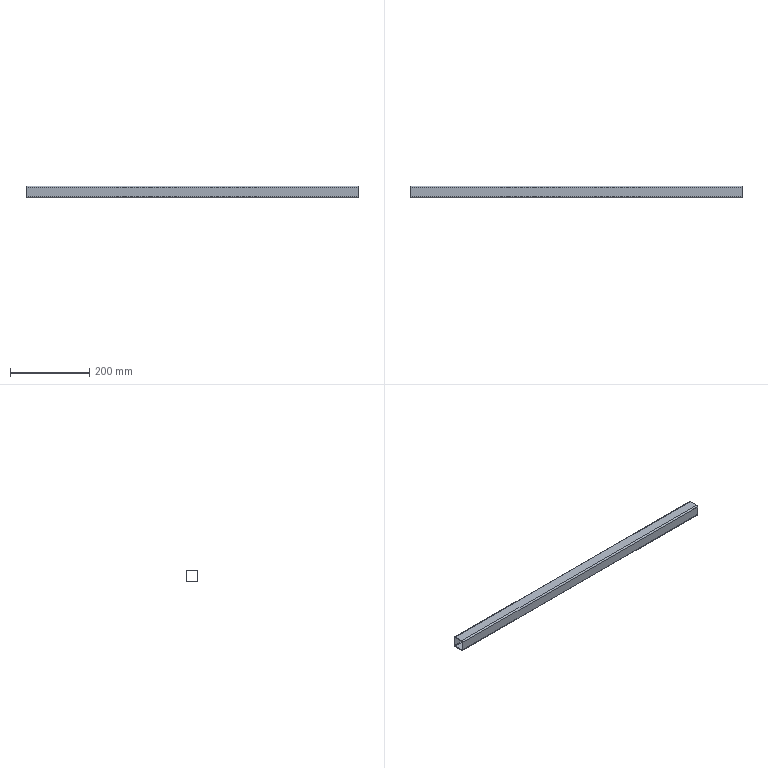Part | SolidWorks | features WeldMemberFeat 1, WeldmentFeature 1 | 1 solid | 18 faces | box 838 x 30 x 30 mm | volume 180231 mm3 | plane 10 | cylinder 8 | commonest cylinder face diameters 3.2 x4 7.2 x4
STEP:
#1=CARTESIAN_POINT('',(-419.,11.4,-15.));
#2=VERTEX_POINT('',#1);
#3=CARTESIAN_POINT('',(-419.,15.,-11.4));
#4=VERTEX_POINT('',#3);
#5=CARTESIAN_POINT('',(-419.,11.4,-11.4));
#6=DIRECTION('',(1.,0.,0.));
#7=DIRECTION('',(0.,0.,-1.));
#8=AXIS2_PLACEMENT_3D('',#5,#6,#7);
#9=CIRCLE('',#8,3.6);
#10=EDGE_CURVE('',#2,#4,#9,.T.);
#11=ORIENTED_EDGE('',*,*,#10,.T.);
#12=CARTESIAN_POINT('',(419.,15.,-11.4));
#13=VERTEX_POINT('',#12);
#14=CARTESIAN_POINT('',(419.,15.,-11.4));
#15=DIRECTION('',(-1.,0.,0.));
#16=VECTOR('',#15,1000.);
#17=LINE('',#14,#16);
#18=EDGE_CURVE('',#13,#4,#17,.T.);
#19=ORIENTED_EDGE('',*,*,#18,.F.);
#20=CARTESIAN_POINT('',(419.,11.4,-15.));
#21=VERTEX_POINT('',#20);
#22=CARTESIAN_POINT('',(419.,11.4,-11.4));
#23=DIRECTION('',(1.,0.,0.));
#24=DIRECTION('',(0.,0.,-1.));
#25=AXIS2_PLACEMENT_3D('',#22,#23,#24);
#26=CIRCLE('',#25,3.6);
#27=EDGE_CURVE('',#21,#13,#26,.T.);
#28=ORIENTED_EDGE('',*,*,#27,.F.);
#29=CARTESIAN_POINT('',(419.,11.4,-15.));
#30=DIRECTION('',(-1.,0.,0.));
#31=VECTOR('',#30,1000.);
#32=LINE('',#29,#31);
#33=EDGE_CURVE('',#21,#2,#32,.T.);
#34=ORIENTED_EDGE('',*,*,#33,.T.);
#35=EDGE_LOOP('',(#11,#19,#28,#34));
#36=FACE_OUTER_BOUND('',#35,.T.);
#37=CARTESIAN_POINT('',(419.,11.4,-11.4));
#38=DIRECTION('',(-1.,0.,0.));
#39=DIRECTION('',(0.,0.,1.));
#40=AXIS2_PLACEMENT_3D('',#37,#38,#39);
#41=CYLINDRICAL_SURFACE('',#40,3.6);
#42=ADVANCED_FACE('',(#36),#41,.T.);
#43=CARTESIAN_POINT('',(-419.,15.,11.4));
#44=VERTEX_POINT('',#43);
#45=CARTESIAN_POINT('',(-419.,15.,-11.4));
#46=DIRECTION('',(0.,0.,1.));
#47=VECTOR('',#46,1000.);
#48=LINE('',#45,#47);
#49=EDGE_CURVE('',#4,#44,#48,.T.);
#50=ORIENTED_EDGE('',*,*,#49,.T.);
#51=CARTESIAN_POINT('',(419.,15.,11.4));
#52=VERTEX_POINT('',#51);
#53=CARTESIAN_POINT('',(419.,15.,11.4));
#54=DIRECTION('',(-1.,0.,0.));
#55=VECTOR('',#54,1000.);
#56=LINE('',#53,#55);
#57=EDGE_CURVE('',#52,#44,#56,.T.);
#58=ORIENTED_EDGE('',*,*,#57,.F.);
#59=CARTESIAN_POINT('',(419.,15.,-11.4));
#60=DIRECTION('',(0.,0.,1.));
#61=VECTOR('',#60,1000.);
#62=LINE('',#59,#61);
#63=EDGE_CURVE('',#13,#52,#62,.T.);
#64=ORIENTED_EDGE('',*,*,#63,.F.);
#65=ORIENTED_EDGE('',*,*,#18,.T.);
#66=EDGE_LOOP('',(#50,#58,#64,#65));
#67=FACE_OUTER_BOUND('',#66,.T.);
#68=CARTESIAN_POINT('',(419.,15.,-11.4));
#69=DIRECTION('',(0.,-1.,0.));
#70=DIRECTION('',(0.,0.,-1.));
#71=AXIS2_PLACEMENT_3D('',#68,#69,#70);
#72=PLANE('',#71);
#73=ADVANCED_FACE('',(#67),#72,.F.);
#74=CARTESIAN_POINT('',(-419.,11.4,15.));
#75=VERTEX_POINT('',#74);
#76=CARTESIAN_POINT('',(-419.,11.4,11.4));
#77=DIRECTION('',(1.,0.,0.));
#78=DIRECTION('',(0.,0.,-1.));
#79=AXIS2_PLACEMENT_3D('',#76,#77,#78);
#80=CIRCLE('',#79,3.6);
#81=EDGE_CURVE('',#44,#75,#80,.T.);
#82=ORIENTED_EDGE('',*,*,#81,.T.);
#83=CARTESIAN_POINT('',(419.,11.4,15.));
#84=VERTEX_POINT('',#83);
#85=CARTESIAN_POINT('',(419.,11.4,15.));
#86=DIRECTION('',(-1.,0.,0.));
#87=VECTOR('',#86,1000.);
#88=LINE('',#85,#87);
#89=EDGE_CURVE('',#84,#75,#88,.T.);
#90=ORIENTED_EDGE('',*,*,#89,.F.);
#91=CARTESIAN_POINT('',(419.,11.4,11.4));
#92=DIRECTION('',(1.,0.,0.));
#93=DIRECTION('',(0.,0.,-1.));
#94=AXIS2_PLACEMENT_3D('',#91,#92,#93);
#95=CIRCLE('',#94,3.6);
#96=EDGE_CURVE('',#52,#84,#95,.T.);
#97=ORIENTED_EDGE('',*,*,#96,.F.);
#98=ORIENTED_EDGE('',*,*,#57,.T.);
#99=EDGE_LOOP('',(#82,#90,#97,#98));
#100=FACE_OUTER_BOUND('',#99,.T.);
#101=CARTESIAN_POINT('',(419.,11.4,11.4));
#102=DIRECTION('',(-1.,0.,0.));
#103=DIRECTION('',(0.,0.,1.));
#104=AXIS2_PLACEMENT_3D('',#101,#102,#103);
#105=CYLINDRICAL_SURFACE('',#104,3.6);
#106=ADVANCED_FACE('',(#100),#105,.T.);
#107=CARTESIAN_POINT('',(-419.,-11.4,15.));
#108=VERTEX_POINT('',#107);
#109=CARTESIAN_POINT('',(-419.,-11.4,15.));
#110=DIRECTION('',(0.,-1.,0.));
#111=VECTOR('',#110,1000.);
#112=LINE('',#109,#111);
#113=EDGE_CURVE('',#75,#108,#112,.T.);
#114=ORIENTED_EDGE('',*,*,#113,.T.);
#115=CARTESIAN_POINT('',(419.,-11.4,15.));
#116=VERTEX_POINT('',#115);
#117=CARTESIAN_POINT('',(419.,-11.4,15.));
#118=DIRECTION('',(-1.,0.,0.));
#119=VECTOR('',#118,1000.);
#120=LINE('',#117,#119);
#121=EDGE_CURVE('',#116,#108,#120,.T.);
#122=ORIENTED_EDGE('',*,*,#121,.F.);
#123=CARTESIAN_POINT('',(419.,-11.4,15.));
#124=DIRECTION('',(0.,-1.,0.));
#125=VECTOR('',#124,1000.);
#126=LINE('',#123,#125);
#127=EDGE_CURVE('',#84,#116,#126,.T.);
#128=ORIENTED_EDGE('',*,*,#127,.F.);
#129=ORIENTED_EDGE('',*,*,#89,.T.);
#130=EDGE_LOOP('',(#114,#122,#128,#129));
#131=FACE_OUTER_BOUND('',#130,.T.);
#132=CARTESIAN_POINT('',(419.,-11.4,15.));
#133=DIRECTION('',(0.,0.,-1.));
#134=DIRECTION('',(-1.,0.,0.));
#135=AXIS2_PLACEMENT_3D('',#132,#133,#134);
#136=PLANE('',#135);
#137=ADVANCED_FACE('',(#131),#136,.F.);
#138=CARTESIAN_POINT('',(-419.,-15.,11.4));
#139=VERTEX_POINT('',#138);
#140=CARTESIAN_POINT('',(-419.,-11.4,11.4));
#141=DIRECTION('',(1.,0.,0.));
#142=DIRECTION('',(0.,0.,-1.));
#143=AXIS2_PLACEMENT_3D('',#140,#141,#142);
#144=CIRCLE('',#143,3.6);
#145=EDGE_CURVE('',#108,#139,#144,.T.);
#146=ORIENTED_EDGE('',*,*,#145,.T.);
#147=CARTESIAN_POINT('',(419.,-15.,11.4));
#148=VERTEX_POINT('',#147);
#149=CARTESIAN_POINT('',(419.,-15.,11.4));
#150=DIRECTION('',(-1.,0.,0.));
#151=VECTOR('',#150,1000.);
#152=LINE('',#149,#151);
#153=EDGE_CURVE('',#148,#139,#152,.T.);
#154=ORIENTED_EDGE('',*,*,#153,.F.);
#155=CARTESIAN_POINT('',(419.,-11.4,11.4));
#156=DIRECTION('',(1.,0.,0.));
#157=DIRECTION('',(0.,0.,-1.));
#158=AXIS2_PLACEMENT_3D('',#155,#156,#157);
#159=CIRCLE('',#158,3.6);
#160=EDGE_CURVE('',#116,#148,#159,.T.);
#161=ORIENTED_EDGE('',*,*,#160,.F.);
#162=ORIENTED_EDGE('',*,*,#121,.T.);
#163=EDGE_LOOP('',(#146,#154,#161,#162));
#164=FACE_OUTER_BOUND('',#163,.T.);
#165=CARTESIAN_POINT('',(419.,-11.4,11.4));
#166=DIRECTION('',(-1.,0.,0.));
#167=DIRECTION('',(0.,0.,1.));
#168=AXIS2_PLACEMENT_3D('',#165,#166,#167);
#169=CYLINDRICAL_SURFACE('',#168,3.6);
#170=ADVANCED_FACE('',(#164),#169,.T.);
#171=CARTESIAN_POINT('',(-419.,-15.,-11.4));
#172=VERTEX_POINT('',#171);
#173=CARTESIAN_POINT('',(-419.,-15.,11.4));
#174=DIRECTION('',(0.,0.,-1.));
#175=VECTOR('',#174,1000.);
#176=LINE('',#173,#175);
#177=EDGE_CURVE('',#139,#172,#176,.T.);
#178=ORIENTED_EDGE('',*,*,#177,.T.);
#179=CARTESIAN_POINT('',(419.,-15.,-11.4));
#180=VERTEX_POINT('',#179);
#181=CARTESIAN_POINT('',(419.,-15.,-11.4));
#182=DIRECTION('',(-1.,0.,0.));
#183=VECTOR('',#182,1000.);
#184=LINE('',#181,#183);
#185=EDGE_CURVE('',#180,#172,#184,.T.);
#186=ORIENTED_EDGE('',*,*,#185,.F.);
#187=CARTESIAN_POINT('',(419.,-15.,11.4));
#188=DIRECTION('',(0.,0.,-1.));
#189=VECTOR('',#188,1000.);
#190=LINE('',#187,#189);
#191=EDGE_CURVE('',#148,#180,#190,.T.);
#192=ORIENTED_EDGE('',*,*,#191,.F.);
#193=ORIENTED_EDGE('',*,*,#153,.T.);
#194=EDGE_LOOP('',(#178,#186,#192,#193));
#195=FACE_OUTER_BOUND('',#194,.T.);
#196=CARTESIAN_POINT('',(419.,-15.,11.4));
#197=DIRECTION('',(0.,1.,0.));
#198=DIRECTION('',(0.,0.,1.));
#199=AXIS2_PLACEMENT_3D('',#196,#197,#198);
#200=PLANE('',#199);
#201=ADVANCED_FACE('',(#195),#200,.F.);
#202=CARTESIAN_POINT('',(-419.,-11.4,-15.));
#203=VERTEX_POINT('',#202);
#204=CARTESIAN_POINT('',(-419.,-11.4,-11.4));
#205=DIRECTION('',(1.,0.,0.));
#206=DIRECTION('',(0.,0.,-1.));
#207=AXIS2_PLACEMENT_3D('',#204,#205,#206);
#208=CIRCLE('',#207,3.6);
#209=EDGE_CURVE('',#172,#203,#208,.T.);
#210=ORIENTED_EDGE('',*,*,#209,.T.);
#211=CARTESIAN_POINT('',(419.,-11.4,-15.));
#212=VERTEX_POINT('',#211);
#213=CARTESIAN_POINT('',(419.,-11.4,-15.));
#214=DIRECTION('',(-1.,0.,0.));
#215=VECTOR('',#214,1000.);
#216=LINE('',#213,#215);
#217=EDGE_CURVE('',#212,#203,#216,.T.);
#218=ORIENTED_EDGE('',*,*,#217,.F.);
#219=CARTESIAN_POINT('',(419.,-11.4,-11.4));
#220=DIRECTION('',(1.,0.,0.));
#221=DIRECTION('',(0.,0.,-1.));
#222=AXIS2_PLACEMENT_3D('',#219,#220,#221);
#223=CIRCLE('',#222,3.6);
#224=EDGE_CURVE('',#180,#212,#223,.T.);
#225=ORIENTED_EDGE('',*,*,#224,.F.);
#226=ORIENTED_EDGE('',*,*,#185,.T.);
#227=EDGE_LOOP('',(#210,#218,#225,#226));
#228=FACE_OUTER_BOUND('',#227,.T.);
#229=CARTESIAN_POINT('',(419.,-11.4,-11.4));
#230=DIRECTION('',(-1.,0.,0.));
#231=DIRECTION('',(0.,0.,1.));
#232=AXIS2_PLACEMENT_3D('',#229,#230,#231);
#233=CYLINDRICAL_SURFACE('',#232,3.6);
#234=ADVANCED_FACE('',(#228),#233,.T.);
#235=CARTESIAN_POINT('',(-419.,13.,11.4));
#236=VERTEX_POINT('',#235);
#237=CARTESIAN_POINT('',(-419.,11.4,13.));
#238=VERTEX_POINT('',#237);
#239=CARTESIAN_POINT('',(-419.,11.4,11.4));
#240=DIRECTION('',(1.,0.,0.));
#241=DIRECTION('',(0.,0.,-1.));
#242=AXIS2_PLACEMENT_3D('',#239,#240,#241);
#243=CIRCLE('',#242,1.6);
#244=EDGE_CURVE('',#236,#238,#243,.T.);
#245=ORIENTED_EDGE('',*,*,#244,.F.);
#246=CARTESIAN_POINT('',(419.,13.,11.4));
#247=VERTEX_POINT('',#246);
#248=CARTESIAN_POINT('',(419.,13.,11.4));
#249=DIRECTION('',(-1.,0.,0.));
#250=VECTOR('',#249,1000.);
#251=LINE('',#248,#250);
#252=EDGE_CURVE('',#247,#236,#251,.T.);
#253=ORIENTED_EDGE('',*,*,#252,.F.);
#254=CARTESIAN_POINT('',(419.,11.4,13.));
#255=VERTEX_POINT('',#254);
#256=CARTESIAN_POINT('',(419.,11.4,11.4));
#257=DIRECTION('',(1.,0.,0.));
#258=DIRECTION('',(0.,0.,-1.));
#259=AXIS2_PLACEMENT_3D('',#256,#257,#258);
#260=CIRCLE('',#259,1.6);
#261=EDGE_CURVE('',#247,#255,#260,.T.);
#262=ORIENTED_EDGE('',*,*,#261,.T.);
#263=CARTESIAN_POINT('',(419.,11.4,13.));
#264=DIRECTION('',(-1.,0.,0.));
#265=VECTOR('',#264,1000.);
#266=LINE('',#263,#265);
#267=EDGE_CURVE('',#255,#238,#266,.T.);
#268=ORIENTED_EDGE('',*,*,#267,.T.);
#269=EDGE_LOOP('',(#245,#253,#262,#268));
#270=FACE_OUTER_BOUND('',#269,.T.);
#271=CARTESIAN_POINT('',(419.,11.4,11.4));
#272=DIRECTION('',(-1.,0.,0.));
#273=DIRECTION('',(0.,0.,1.));
#274=AXIS2_PLACEMENT_3D('',#271,#272,#273);
#275=CYLINDRICAL_SURFACE('',#274,1.6);
#276=ADVANCED_FACE('',(#270),#275,.F.);
#277=CARTESIAN_POINT('',(-419.,13.,-11.4));
#278=VERTEX_POINT('',#277);
#279=CARTESIAN_POINT('',(-419.,13.,-11.4));
#280=DIRECTION('',(0.,0.,1.));
#281=VECTOR('',#280,1000.);
#282=LINE('',#279,#281);
#283=EDGE_CURVE('',#278,#236,#282,.T.);
#284=ORIENTED_EDGE('',*,*,#283,.F.);
#285=CARTESIAN_POINT('',(419.,13.,-11.4));
#286=VERTEX_POINT('',#285);
#287=CARTESIAN_POINT('',(419.,13.,-11.4));
#288=DIRECTION('',(-1.,0.,0.));
#289=VECTOR('',#288,1000.);
#290=LINE('',#287,#289);
#291=EDGE_CURVE('',#286,#278,#290,.T.);
#292=ORIENTED_EDGE('',*,*,#291,.F.);
#293=CARTESIAN_POINT('',(419.,13.,-11.4));
#294=DIRECTION('',(0.,0.,1.));
#295=VECTOR('',#294,1000.);
#296=LINE('',#293,#295);
#297=EDGE_CURVE('',#286,#247,#296,.T.);
#298=ORIENTED_EDGE('',*,*,#297,.T.);
#299=ORIENTED_EDGE('',*,*,#252,.T.);
#300=EDGE_LOOP('',(#284,#292,#298,#299));
#301=FACE_OUTER_BOUND('',#300,.T.);
#302=CARTESIAN_POINT('',(419.,13.,-11.4));
#303=DIRECTION('',(0.,-1.,0.));
#304=DIRECTION('',(0.,0.,-1.));
#305=AXIS2_PLACEMENT_3D('',#302,#303,#304);
#306=PLANE('',#305);
#307=ADVANCED_FACE('',(#301),#306,.T.);
#308=CARTESIAN_POINT('',(-419.,11.4,-13.));
#309=VERTEX_POINT('',#308);
#310=CARTESIAN_POINT('',(-419.,11.4,-11.4));
#311=DIRECTION('',(1.,0.,0.));
#312=DIRECTION('',(0.,0.,-1.));
#313=AXIS2_PLACEMENT_3D('',#310,#311,#312);
#314=CIRCLE('',#313,1.6);
#315=EDGE_CURVE('',#309,#278,#314,.T.);
#316=ORIENTED_EDGE('',*,*,#315,.F.);
#317=CARTESIAN_POINT('',(419.,11.4,-13.));
#318=VERTEX_POINT('',#317);
#319=CARTESIAN_POINT('',(419.,11.4,-13.));
#320=DIRECTION('',(-1.,0.,0.));
#321=VECTOR('',#320,1000.);
#322=LINE('',#319,#321);
#323=EDGE_CURVE('',#318,#309,#322,.T.);
#324=ORIENTED_EDGE('',*,*,#323,.F.);
#325=CARTESIAN_POINT('',(419.,11.4,-11.4));
#326=DIRECTION('',(1.,0.,0.));
#327=DIRECTION('',(0.,0.,-1.));
#328=AXIS2_PLACEMENT_3D('',#325,#326,#327);
#329=CIRCLE('',#328,1.6);
#330=EDGE_CURVE('',#318,#286,#329,.T.);
#331=ORIENTED_EDGE('',*,*,#330,.T.);
#332=ORIENTED_EDGE('',*,*,#291,.T.);
#333=EDGE_LOOP('',(#316,#324,#331,#332));
#334=FACE_OUTER_BOUND('',#333,.T.);
#335=CARTESIAN_POINT('',(419.,11.4,-11.4));
#336=DIRECTION('',(-1.,0.,0.));
#337=DIRECTION('',(0.,0.,1.));
#338=AXIS2_PLACEMENT_3D('',#335,#336,#337);
#339=CYLINDRICAL_SURFACE('',#338,1.6);
#340=ADVANCED_FACE('',(#334),#339,.F.);
#341=CARTESIAN_POINT('',(-419.,-11.4,-13.));
#342=VERTEX_POINT('',#341);
#343=CARTESIAN_POINT('',(-419.,11.4,-13.));
#344=DIRECTION('',(0.,1.,0.));
#345=VECTOR('',#344,1000.);
#346=LINE('',#343,#345);
#347=EDGE_CURVE('',#342,#309,#346,.T.);
#348=ORIENTED_EDGE('',*,*,#347,.F.);
#349=CARTESIAN_POINT('',(419.,-11.4,-13.));
#350=VERTEX_POINT('',#349);
#351=CARTESIAN_POINT('',(419.,-11.4,-13.));
#352=DIRECTION('',(-1.,0.,0.));
#353=VECTOR('',#352,1000.);
#354=LINE('',#351,#353);
#355=EDGE_CURVE('',#350,#342,#354,.T.);
#356=ORIENTED_EDGE('',*,*,#355,.F.);
#357=CARTESIAN_POINT('',(419.,11.4,-13.));
#358=DIRECTION('',(0.,1.,0.));
#359=VECTOR('',#358,1000.);
#360=LINE('',#357,#359);
#361=EDGE_CURVE('',#350,#318,#360,.T.);
#362=ORIENTED_EDGE('',*,*,#361,.T.);
#363=ORIENTED_EDGE('',*,*,#323,.T.);
#364=EDGE_LOOP('',(#348,#356,#362,#363));
#365=FACE_OUTER_BOUND('',#364,.T.);
#366=CARTESIAN_POINT('',(419.,11.4,-13.));
#367=DIRECTION('',(0.,0.,1.));
#368=DIRECTION('',(1.,0.,0.));
#369=AXIS2_PLACEMENT_3D('',#366,#367,#368);
#370=PLANE('',#369);
#371=ADVANCED_FACE('',(#365),#370,.T.);
#372=CARTESIAN_POINT('',(-419.,-13.,-11.4));
#373=VERTEX_POINT('',#372);
#374=CARTESIAN_POINT('',(-419.,-11.4,-11.4));
#375=DIRECTION('',(1.,0.,0.));
#376=DIRECTION('',(0.,0.,-1.));
#377=AXIS2_PLACEMENT_3D('',#374,#375,#376);
#378=CIRCLE('',#377,1.6);
#379=EDGE_CURVE('',#373,#342,#378,.T.);
#380=ORIENTED_EDGE('',*,*,#379,.F.);
#381=CARTESIAN_POINT('',(419.,-13.,-11.4));
#382=VERTEX_POINT('',#381);
#383=CARTESIAN_POINT('',(419.,-13.,-11.4));
#384=DIRECTION('',(-1.,0.,0.));
#385=VECTOR('',#384,1000.);
#386=LINE('',#383,#385);
#387=EDGE_CURVE('',#382,#373,#386,.T.);
#388=ORIENTED_EDGE('',*,*,#387,.F.);
#389=CARTESIAN_POINT('',(419.,-11.4,-11.4));
#390=DIRECTION('',(1.,0.,0.));
#391=DIRECTION('',(0.,0.,-1.));
#392=AXIS2_PLACEMENT_3D('',#389,#390,#391);
#393=CIRCLE('',#392,1.6);
#394=EDGE_CURVE('',#382,#350,#393,.T.);
#395=ORIENTED_EDGE('',*,*,#394,.T.);
#396=ORIENTED_EDGE('',*,*,#355,.T.);
#397=EDGE_LOOP('',(#380,#388,#395,#396));
#398=FACE_OUTER_BOUND('',#397,.T.);
#399=CARTESIAN_POINT('',(419.,-11.4,-11.4));
#400=DIRECTION('',(-1.,0.,0.));
#401=DIRECTION('',(0.,0.,1.));
#402=AXIS2_PLACEMENT_3D('',#399,#400,#401);
#403=CYLINDRICAL_SURFACE('',#402,1.6);
#404=ADVANCED_FACE('',(#398),#403,.F.);
#405=CARTESIAN_POINT('',(-419.,-13.,11.4));
#406=VERTEX_POINT('',#405);
#407=CARTESIAN_POINT('',(-419.,-13.,11.4));
#408=DIRECTION('',(0.,0.,-1.));
#409=VECTOR('',#408,1000.);
#410=LINE('',#407,#409);
#411=EDGE_CURVE('',#406,#373,#410,.T.);
#412=ORIENTED_EDGE('',*,*,#411,.F.);
#413=CARTESIAN_POINT('',(419.,-13.,11.4));
#414=VERTEX_POINT('',#413);
#415=CARTESIAN_POINT('',(419.,-13.,11.4));
#416=DIRECTION('',(-1.,0.,0.));
#417=VECTOR('',#416,1000.);
#418=LINE('',#415,#417);
#419=EDGE_CURVE('',#414,#406,#418,.T.);
#420=ORIENTED_EDGE('',*,*,#419,.F.);
#421=CARTESIAN_POINT('',(419.,-13.,11.4));
#422=DIRECTION('',(0.,0.,-1.));
#423=VECTOR('',#422,1000.);
#424=LINE('',#421,#423);
#425=EDGE_CURVE('',#414,#382,#424,.T.);
#426=ORIENTED_EDGE('',*,*,#425,.T.);
#427=ORIENTED_EDGE('',*,*,#387,.T.);
#428=EDGE_LOOP('',(#412,#420,#426,#427));
#429=FACE_OUTER_BOUND('',#428,.T.);
#430=CARTESIAN_POINT('',(419.,-13.,11.4));
#431=DIRECTION('',(0.,1.,0.));
#432=DIRECTION('',(0.,0.,1.));
#433=AXIS2_PLACEMENT_3D('',#430,#431,#432);
#434=PLANE('',#433);
#435=ADVANCED_FACE('',(#429),#434,.T.);
#436=CARTESIAN_POINT('',(-419.,-11.4,13.));
#437=VERTEX_POINT('',#436);
#438=CARTESIAN_POINT('',(-419.,-11.4,11.4));
#439=DIRECTION('',(1.,0.,0.));
#440=DIRECTION('',(0.,0.,-1.));
#441=AXIS2_PLACEMENT_3D('',#438,#439,#440);
#442=CIRCLE('',#441,1.6);
#443=EDGE_CURVE('',#437,#406,#442,.T.);
#444=ORIENTED_EDGE('',*,*,#443,.F.);
#445=CARTESIAN_POINT('',(419.,-11.4,13.));
#446=VERTEX_POINT('',#445);
#447=CARTESIAN_POINT('',(419.,-11.4,13.));
#448=DIRECTION('',(-1.,0.,0.));
#449=VECTOR('',#448,1000.);
#450=LINE('',#447,#449);
#451=EDGE_CURVE('',#446,#437,#450,.T.);
#452=ORIENTED_EDGE('',*,*,#451,.F.);
#453=CARTESIAN_POINT('',(419.,-11.4,11.4));
#454=DIRECTION('',(1.,0.,0.));
#455=DIRECTION('',(0.,0.,-1.));
#456=AXIS2_PLACEMENT_3D('',#453,#454,#455);
#457=CIRCLE('',#456,1.6);
#458=EDGE_CURVE('',#446,#414,#457,.T.);
#459=ORIENTED_EDGE('',*,*,#458,.T.);
#460=ORIENTED_EDGE('',*,*,#419,.T.);
#461=EDGE_LOOP('',(#444,#452,#459,#460));
#462=FACE_OUTER_BOUND('',#461,.T.);
#463=CARTESIAN_POINT('',(419.,-11.4,11.4));
#464=DIRECTION('',(-1.,0.,0.));
#465=DIRECTION('',(0.,0.,1.));
#466=AXIS2_PLACEMENT_3D('',#463,#464,#465);
#467=CYLINDRICAL_SURFACE('',#466,1.6);
#468=ADVANCED_FACE('',(#462),#467,.F.);
#469=CARTESIAN_POINT('',(-419.,-11.4,13.));
#470=DIRECTION('',(0.,-1.,0.));
#471=VECTOR('',#470,1000.);
#472=LINE('',#469,#471);
#473=EDGE_CURVE('',#238,#437,#472,.T.);
#474=ORIENTED_EDGE('',*,*,#473,.F.);
#475=ORIENTED_EDGE('',*,*,#267,.F.);
#476=CARTESIAN_POINT('',(419.,-11.4,13.));
#477=DIRECTION('',(0.,-1.,0.));
#478=VECTOR('',#477,1000.);
#479=LINE('',#476,#478);
#480=EDGE_CURVE('',#255,#446,#479,.T.);
#481=ORIENTED_EDGE('',*,*,#480,.T.);
#482=ORIENTED_EDGE('',*,*,#451,.T.);
#483=EDGE_LOOP('',(#474,#475,#481,#482));
#484=FACE_OUTER_BOUND('',#483,.T.);
#485=CARTESIAN_POINT('',(419.,-11.4,13.));
#486=DIRECTION('',(0.,0.,-1.));
#487=DIRECTION('',(-1.,0.,0.));
#488=AXIS2_PLACEMENT_3D('',#485,#486,#487);
#489=PLANE('',#488);
#490=ADVANCED_FACE('',(#484),#489,.T.);
#491=CARTESIAN_POINT('',(-419.,11.4,-15.));
#492=DIRECTION('',(0.,1.,0.));
#493=VECTOR('',#492,1000.);
#494=LINE('',#491,#493);
#495=EDGE_CURVE('',#203,#2,#494,.T.);
#496=ORIENTED_EDGE('',*,*,#495,.T.);
#497=ORIENTED_EDGE('',*,*,#33,.F.);
#498=CARTESIAN_POINT('',(419.,11.4,-15.));
#499=DIRECTION('',(0.,1.,0.));
#500=VECTOR('',#499,1000.);
#501=LINE('',#498,#500);
#502=EDGE_CURVE('',#212,#21,#501,.T.);
#503=ORIENTED_EDGE('',*,*,#502,.F.);
#504=ORIENTED_EDGE('',*,*,#217,.T.);
#505=EDGE_LOOP('',(#496,#497,#503,#504));
#506=FACE_OUTER_BOUND('',#505,.T.);
#507=CARTESIAN_POINT('',(419.,11.4,-15.));
#508=DIRECTION('',(0.,0.,1.));
#509=DIRECTION('',(1.,0.,0.));
#510=AXIS2_PLACEMENT_3D('',#507,#508,#509);
#511=PLANE('',#510);
#512=ADVANCED_FACE('',(#506),#511,.F.);
#513=ORIENTED_EDGE('',*,*,#261,.F.);
#514=ORIENTED_EDGE('',*,*,#297,.F.);
#515=ORIENTED_EDGE('',*,*,#330,.F.);
#516=ORIENTED_EDGE('',*,*,#361,.F.);
#517=ORIENTED_EDGE('',*,*,#394,.F.);
#518=ORIENTED_EDGE('',*,*,#425,.F.);
#519=ORIENTED_EDGE('',*,*,#458,.F.);
#520=ORIENTED_EDGE('',*,*,#480,.F.);
#521=EDGE_LOOP('',(#513,#514,#515,#516,#517,#518,#519,#520));
#522=FACE_BOUND('',#521,.T.);
#523=ORIENTED_EDGE('',*,*,#27,.T.);
#524=ORIENTED_EDGE('',*,*,#63,.T.);
#525=ORIENTED_EDGE('',*,*,#96,.T.);
#526=ORIENTED_EDGE('',*,*,#127,.T.);
#527=ORIENTED_EDGE('',*,*,#160,.T.);
#528=ORIENTED_EDGE('',*,*,#191,.T.);
#529=ORIENTED_EDGE('',*,*,#224,.T.);
#530=ORIENTED_EDGE('',*,*,#502,.T.);
#531=EDGE_LOOP('',(#523,#524,#525,#526,#527,#528,#529,#530));
#532=FACE_OUTER_BOUND('',#531,.T.);
#533=CARTESIAN_POINT('',(419.,11.4,-11.4));
#534=DIRECTION('',(1.,0.,0.));
#535=DIRECTION('',(0.,0.,-1.));
#536=AXIS2_PLACEMENT_3D('',#533,#534,#535);
#537=PLANE('',#536);
#538=ADVANCED_FACE('',(#522,#532),#537,.T.);
#539=ORIENTED_EDGE('',*,*,#244,.T.);
#540=ORIENTED_EDGE('',*,*,#473,.T.);
#541=ORIENTED_EDGE('',*,*,#443,.T.);
#542=ORIENTED_EDGE('',*,*,#411,.T.);
#543=ORIENTED_EDGE('',*,*,#379,.T.);
#544=ORIENTED_EDGE('',*,*,#347,.T.);
#545=ORIENTED_EDGE('',*,*,#315,.T.);
#546=ORIENTED_EDGE('',*,*,#283,.T.);
#547=EDGE_LOOP('',(#539,#540,#541,#542,#543,#544,#545,#546));
#548=FACE_BOUND('',#547,.T.);
#549=ORIENTED_EDGE('',*,*,#10,.F.);
#550=ORIENTED_EDGE('',*,*,#495,.F.);
#551=ORIENTED_EDGE('',*,*,#209,.F.);
#552=ORIENTED_EDGE('',*,*,#177,.F.);
#553=ORIENTED_EDGE('',*,*,#145,.F.);
#554=ORIENTED_EDGE('',*,*,#113,.F.);
#555=ORIENTED_EDGE('',*,*,#81,.F.);
#556=ORIENTED_EDGE('',*,*,#49,.F.);
#557=EDGE_LOOP('',(#549,#550,#551,#552,#553,#554,#555,#556));
#558=FACE_OUTER_BOUND('',#557,.T.);
#559=CARTESIAN_POINT('',(-419.,11.4,-11.4));
#560=DIRECTION('',(1.,0.,0.));
#561=DIRECTION('',(0.,0.,-1.));
#562=AXIS2_PLACEMENT_3D('',#559,#560,#561);
#563=PLANE('',#562);
#564=ADVANCED_FACE('',(#548,#558),#563,.F.);
#565=CLOSED_SHELL('',(#42,#73,#106,#137,#170,#201,#234,#276,#307,#340,#371,#404,#435,#468,#490,#512,#538,#564));
#566=MANIFOLD_SOLID_BREP('',#565);
#567=CARTESIAN_POINT('',(0.,0.,0.));
#568=DIRECTION('',(0.,0.,1.));
#569=DIRECTION('',(1.,0.,0.));
#570=AXIS2_PLACEMENT_3D('',#567,#568,#569);
#571=(LENGTH_UNIT()NAMED_UNIT(*)SI_UNIT(.MILLI.,.METRE.));
#572=UNCERTAINTY_MEASURE_WITH_UNIT(LENGTH_MEASURE(0.00001),#571,'','');
#573=(NAMED_UNIT(*)PLANE_ANGLE_UNIT()SI_UNIT($,.RADIAN.));
#574=(NAMED_UNIT(*)SI_UNIT($,.STERADIAN.)SOLID_ANGLE_UNIT());
#575=(GEOMETRIC_REPRESENTATION_CONTEXT(3)GLOBAL_UNCERTAINTY_ASSIGNED_CONTEXT((#572))GLOBAL_UNIT_ASSIGNED_CONTEXT((#571,#573,#574))REPRESENTATION_CONTEXT('',''));
#576=ADVANCED_BREP_SHAPE_REPRESENTATION('',(#566,#570),#575);